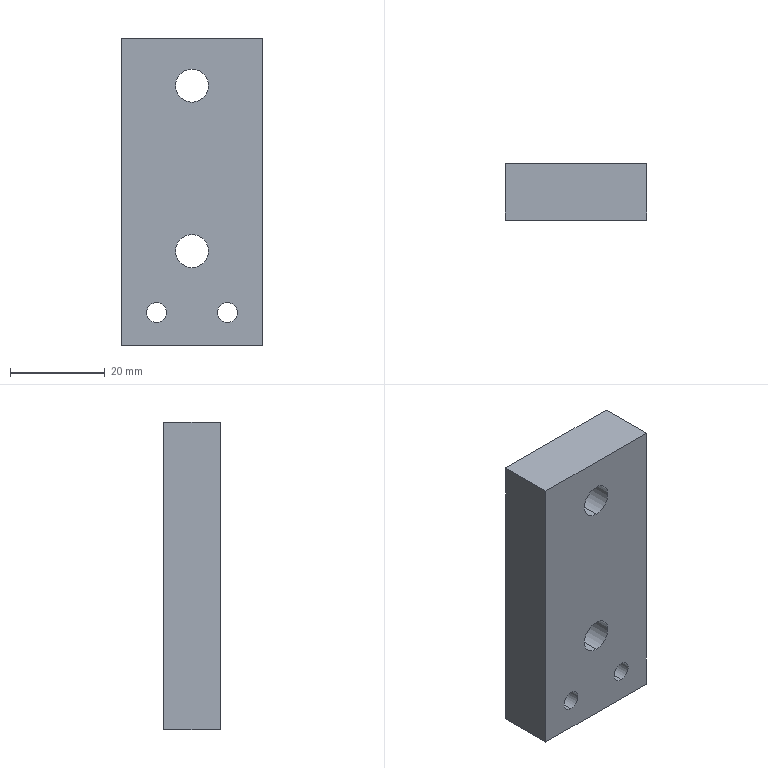Part | STEP file | secondary slingshot input support plate | 1 solid | 20 faces | box 30 x 12 x 65 mm | volume 21465 mm3 | cylinder 12 | plane 8 | commonest cylinder face diameters 4.2 x4 7 x4 11 x4